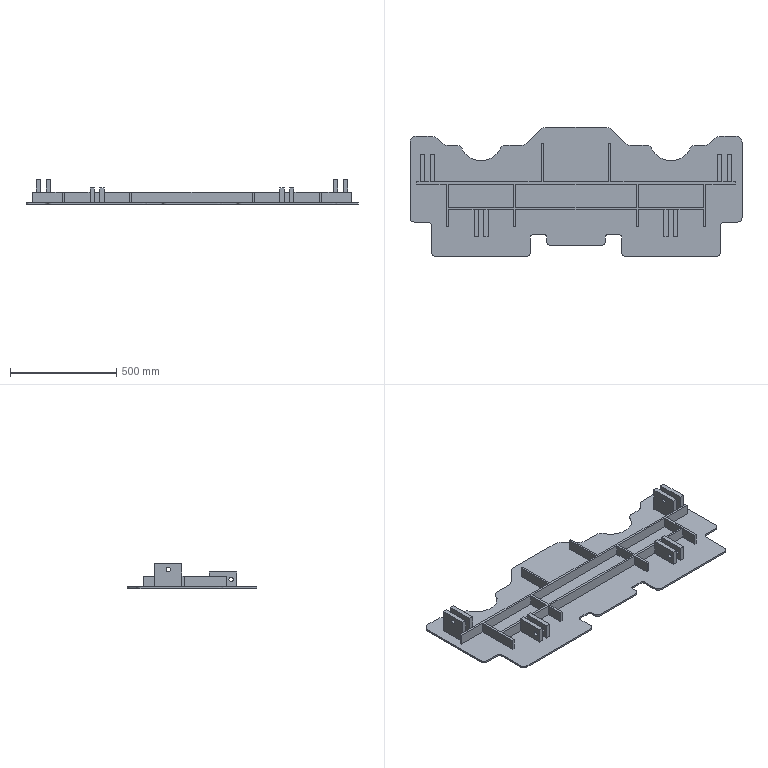Part | NX | features 脚踏板 2 | 1 solid | 158 faces | box 1560 x 608.47 x 118 mm | volume 9927777 mm3 | plane 120 | cylinder 38 | commonest cylinder face diameters 20 x12 40 x10 80 x8 60 x6 197.776 x2